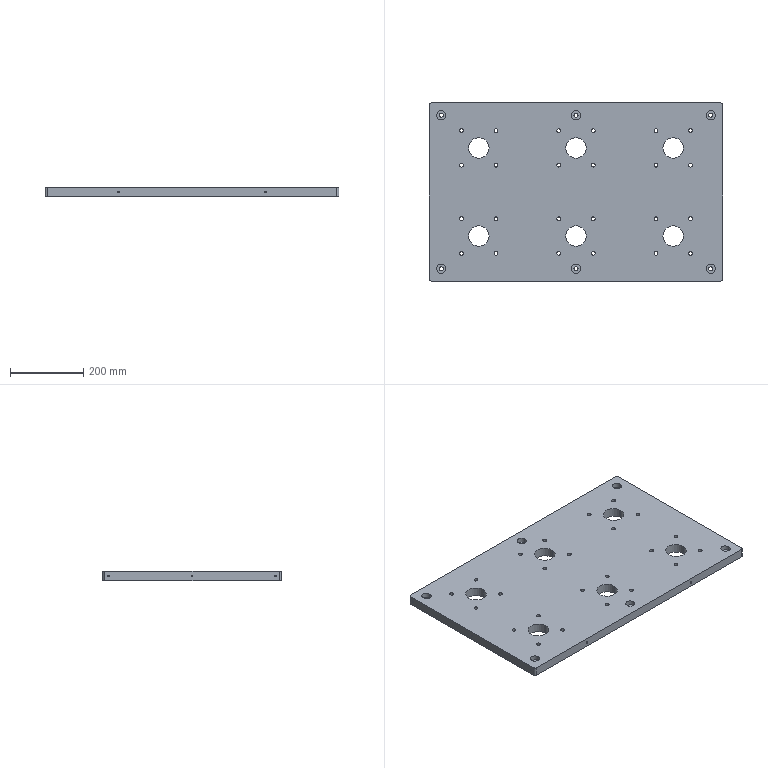Part | 1 solid | 130 faces | box 800 x 485 x 25 mm | volume 9228255 mm3 | cylinder 108 | plane 22 | commonest cylinder face diameters 10.5 x48 5.2 x20 11 x12 25 x12 56 x12 10 x4